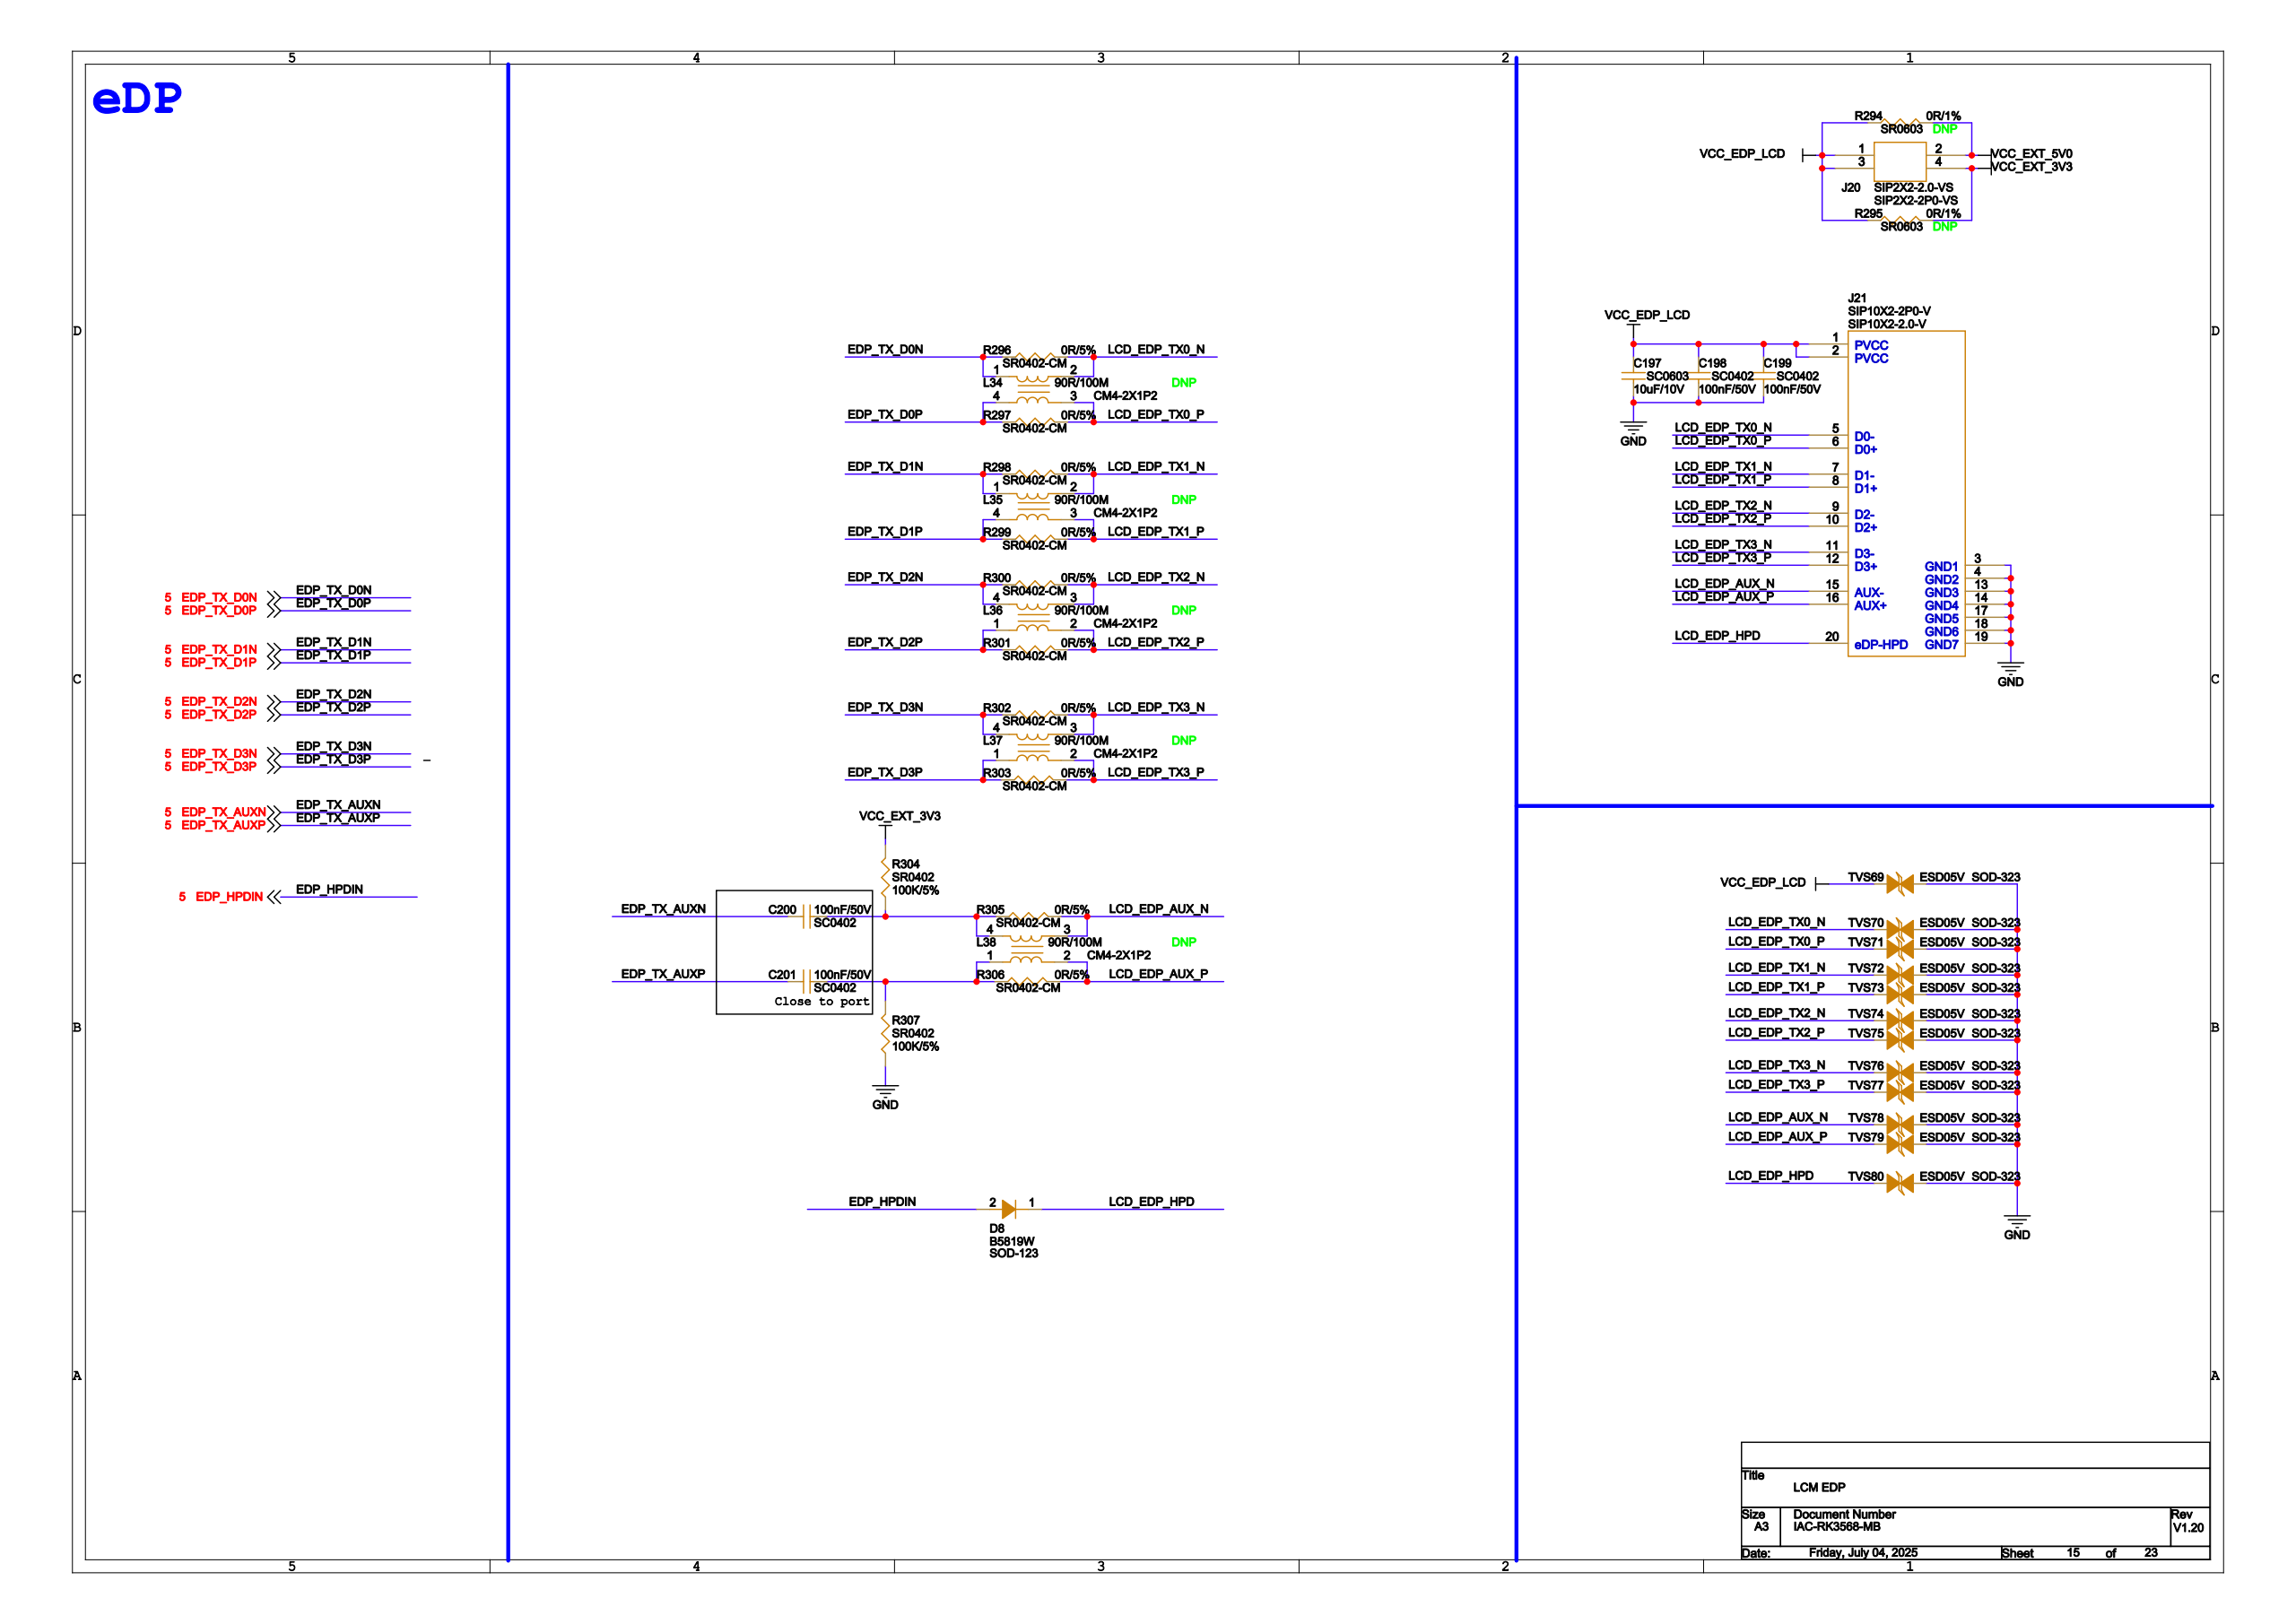Circuit board | Cadence Allegro | 1138 parts | 722 nets | one sheet of the schematic
Parts on this sheet (reference | value | footprint):
C197 | 10uF/10V | SC0603
C198 | 100nF/50V | SC0402
C199 | 100nF/50V | SC0402
C200 | 100nF/50V | SC0402
C201 | 100nF/50V | SC0402
D8 | B5819W | SOD-123
J20 | SIP2X2-2.0-VS | SIP2X2-2P0-VS
J21 | SIP10X2-2.0-V | SIP10X2-2P0-V
L34 | 90R/100M | CM4-2X1P2
L35 | 90R/100M | CM4-2X1P2
L36 | 90R/100M | CM4-2X1P2
L37 | 90R/100M | CM4-2X1P2
L38 | 90R/100M | CM4-2X1P2
R294 | 0R/1% | SR0603
R295 | 0R/1% | SR0603
R296 | 0R/5% | SR0402-CM
R297 | 0R/5% | SR0402-CM
R298 | 0R/5% | SR0402-CM
R299 | 0R/5% | SR0402-CM
R300 | 0R/5% | SR0402-CM
R301 | 0R/5% | SR0402-CM
R302 | 0R/5% | SR0402-CM
R303 | 0R/5% | SR0402-CM
R304 | 100K/5% | SR0402
R305 | 0R/5% | SR0402-CM
R306 | 0R/5% | SR0402-CM
R307 | 100K/5% | SR0402
TVS69 | ESD05V | SOD-323
TVS70 | ESD05V | SOD-323
TVS71 | ESD05V | SOD-323
TVS72 | ESD05V | SOD-323
TVS73 | ESD05V | SOD-323
TVS74 | ESD05V | SOD-323
TVS75 | ESD05V | SOD-323
TVS76 | ESD05V | SOD-323
TVS77 | ESD05V | SOD-323
TVS78 | ESD05V | SOD-323
TVS79 | ESD05V | SOD-323
TVS80 | ESD05V | SOD-323
Nets of these parts (net: part-pin ...):
VCC_EXT_5V0: J20-2 R294-2
EDP_HPDIN: D8-2
LCD_EDP_HPD: D8-1 J21-20 TVS80-1
VCC_EXT_3V3: J20-4 R295-2 R304-2
GND: C197-2 C198-2 C199-2 J21-3 J21-4 J21-13 J21-14 J21-17 J21-18 J21-19 R307-1 TVS69-2 TVS70-2 TVS71-2 TVS72-2 TVS73-2 TVS74-2 TVS75-2 TVS76-2 TVS77-2 TVS78-2 TVS79-2 TVS80-2
VCC_EDP_LCD: C197-1 C198-1 C199-1 J20-1 J20-3 J21-1 J21-2 R294-1 R295-1 TVS69-1
LCD_EDP_TX0_N: J21-5 L34-2 R296-2 TVS70-1
LCD_EDP_TX0_P: J21-6 L34-3 R297-2 TVS71-1
LCD_EDP_TX1_N: J21-7 L35-2 R298-2 TVS72-1
LCD_EDP_TX1_P: J21-8 L35-3 R299-2 TVS73-1
LCD_EDP_TX2_N: J21-9 L36-3 R300-2 TVS74-1
LCD_EDP_TX2_P: J21-10 L36-2 R301-2 TVS75-1
LCD_EDP_TX3_N: J21-11 L37-3 R302-2 TVS76-1
LCD_EDP_TX3_P: J21-12 L37-2 R303-2 TVS77-1
LCD_EDP_AUX_N: J21-15 L38-3 R305-2 TVS78-1
LCD_EDP_AUX_P: J21-16 L38-2 R306-2 TVS79-1
EDP_TX_D0N: L34-1 R296-1
EDP_TX_D0P: L34-4 R297-1
EDP_TX_D1N: L35-1 R298-1
EDP_TX_D1P: L35-4 R299-1
EDP_TX_D2N: L36-4 R300-1
EDP_TX_D2P: L36-1 R301-1
EDP_TX_D3N: L37-4 R302-1
EDP_TX_D3P: L37-1 R303-1
N19578434: C200-2 L38-4 R304-1 R305-1
N19578400: C201-2 L38-1 R306-1 R307-2
EDP_TX_AUXN: C200-1
EDP_TX_AUXP: C201-1